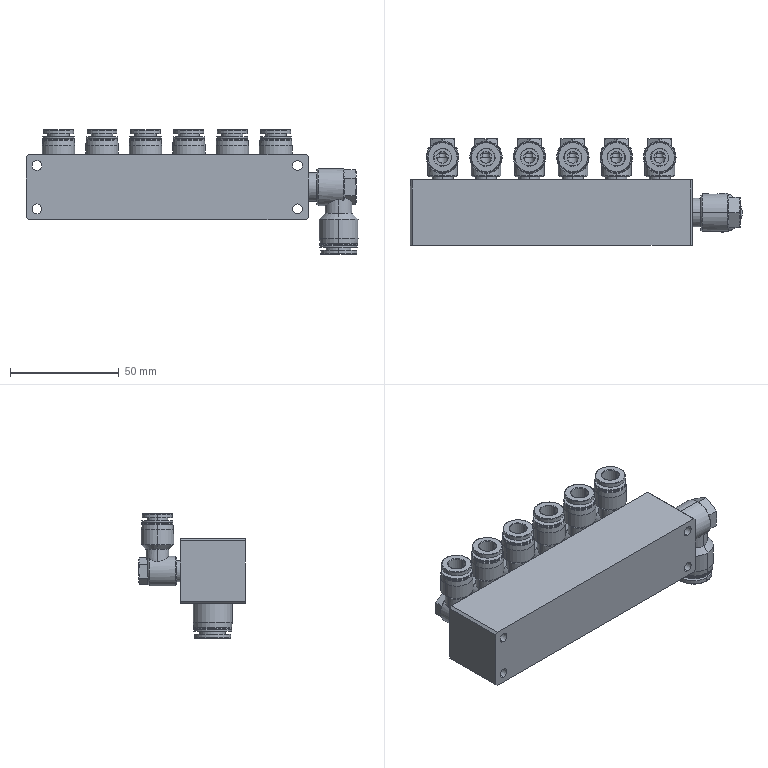Part | SolidWorks | features ReferencePattern 5, DerivedHolePattern 1 | 8 solids | 577 faces | box 152.95 x 49 x 57.5 mm | volume 133914 mm3 | cylinder 191 | plane 182 | cone 155 | spline 49 | commonest cylinder face diameters 14.4 x24 8 x20 4.864 x12 5.333 x12 7.9 x12 9.728 x12